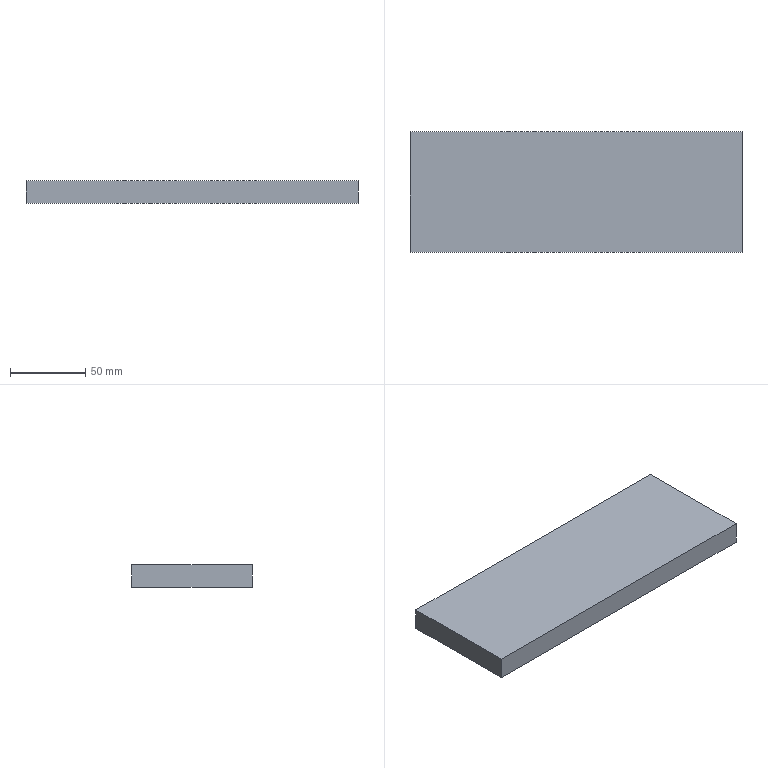Part | STEP file | Tube feed_id586_x_t | 1 solid | 6 faces | box 220 x 80 x 15 mm | volume 264000 mm3 | plane 6
STEP:
#1=CARTESIAN_POINT('',(0.,0.,0.));
#2=DIRECTION('',(0.,0.,1.));
#3=DIRECTION('',(1.,0.,0.));
#4=AXIS2_PLACEMENT_3D('',#1,#2,#3);
#5=CARTESIAN_POINT('',(21.,250.936,-219.));
#6=VERTEX_POINT('',#5);
#7=CARTESIAN_POINT('',(21.,170.936,-219.));
#8=VERTEX_POINT('',#7);
#9=CARTESIAN_POINT('',(21.,250.936,-219.));
#10=DIRECTION('',(0.,-1.,0.));
#11=VECTOR('',#10,1.);
#12=LINE('',#9,#11);
#13=CARTESIAN_POINT('',(21.,250.936,-204.));
#14=DIRECTION('',(1.,0.,0.));
#15=DIRECTION('',(0.,0.,-1.));
#16=AXIS2_PLACEMENT_3D('',#13,#14,#15);
#17=PLANE('',#16);
#18=CARTESIAN_POINT('',(15.,0.));
#19=DIRECTION('',(0.,-1.));
#20=VECTOR('',#19,1.);
#21=LINE('',#18,#20);
#22=(GEOMETRIC_REPRESENTATION_CONTEXT(2)PARAMETRIC_REPRESENTATION_CONTEXT()REPRESENTATION_CONTEXT('',''));
#23=DEFINITIONAL_REPRESENTATION('',(#21),#22);
#24=PCURVE('',#17,#23);
#25=CARTESIAN_POINT('',(0.,0.,-219.));
#26=DIRECTION('',(0.,0.,1.));
#27=DIRECTION('',(1.,0.,0.));
#28=AXIS2_PLACEMENT_3D('',#25,#26,#27);
#29=PLANE('',#28);
#30=CARTESIAN_POINT('',(21.,250.936));
#31=DIRECTION('',(0.,-1.));
#32=VECTOR('',#31,1.);
#33=LINE('',#30,#32);
#34=(GEOMETRIC_REPRESENTATION_CONTEXT(2)PARAMETRIC_REPRESENTATION_CONTEXT()REPRESENTATION_CONTEXT('',''));
#35=DEFINITIONAL_REPRESENTATION('',(#33),#34);
#36=PCURVE('',#29,#35);
#37=SURFACE_CURVE('',#12,(#24,#36),.PCURVE_S1.);
#38=EDGE_CURVE('',#6,#8,#37,.T.);
#39=ORIENTED_EDGE('',*,*,#38,.T.);
#40=CARTESIAN_POINT('',(21.,170.936,-204.));
#41=VERTEX_POINT('',#40);
#42=CARTESIAN_POINT('',(21.,170.936,-204.));
#43=DIRECTION('',(0.,0.,-1.));
#44=VECTOR('',#43,1.);
#45=LINE('',#42,#44);
#46=CARTESIAN_POINT('',(0.,-80.));
#47=DIRECTION('',(1.,0.));
#48=VECTOR('',#47,1.);
#49=LINE('',#46,#48);
#50=(GEOMETRIC_REPRESENTATION_CONTEXT(2)PARAMETRIC_REPRESENTATION_CONTEXT()REPRESENTATION_CONTEXT('',''));
#51=DEFINITIONAL_REPRESENTATION('',(#49),#50);
#52=PCURVE('',#17,#51);
#53=CARTESIAN_POINT('',(21.,170.936,-204.));
#54=DIRECTION('',(0.,1.,0.));
#55=DIRECTION('',(0.,0.,1.));
#56=AXIS2_PLACEMENT_3D('',#53,#54,#55);
#57=PLANE('',#56);
#58=CARTESIAN_POINT('',(0.,0.));
#59=DIRECTION('',(-1.,0.));
#60=VECTOR('',#59,1.);
#61=LINE('',#58,#60);
#62=(GEOMETRIC_REPRESENTATION_CONTEXT(2)PARAMETRIC_REPRESENTATION_CONTEXT()REPRESENTATION_CONTEXT('',''));
#63=DEFINITIONAL_REPRESENTATION('',(#61),#62);
#64=PCURVE('',#57,#63);
#65=SURFACE_CURVE('',#45,(#52,#64),.PCURVE_S1.);
#66=EDGE_CURVE('',#41,#8,#65,.T.);
#67=ORIENTED_EDGE('',*,*,#66,.F.);
#68=CARTESIAN_POINT('',(21.,250.936,-204.));
#69=VERTEX_POINT('',#68);
#70=CARTESIAN_POINT('',(21.,250.936,-204.));
#71=DIRECTION('',(0.,-1.,0.));
#72=VECTOR('',#71,1.);
#73=LINE('',#70,#72);
#74=CARTESIAN_POINT('',(0.,0.));
#75=DIRECTION('',(0.,-1.));
#76=VECTOR('',#75,1.);
#77=LINE('',#74,#76);
#78=(GEOMETRIC_REPRESENTATION_CONTEXT(2)PARAMETRIC_REPRESENTATION_CONTEXT()REPRESENTATION_CONTEXT('',''));
#79=DEFINITIONAL_REPRESENTATION('',(#77),#78);
#80=PCURVE('',#17,#79);
#81=CARTESIAN_POINT('',(0.,0.,-204.));
#82=DIRECTION('',(0.,0.,1.));
#83=DIRECTION('',(1.,0.,0.));
#84=AXIS2_PLACEMENT_3D('',#81,#82,#83);
#85=PLANE('',#84);
#86=CARTESIAN_POINT('',(21.,250.936));
#87=DIRECTION('',(0.,-1.));
#88=VECTOR('',#87,1.);
#89=LINE('',#86,#88);
#90=(GEOMETRIC_REPRESENTATION_CONTEXT(2)PARAMETRIC_REPRESENTATION_CONTEXT()REPRESENTATION_CONTEXT('',''));
#91=DEFINITIONAL_REPRESENTATION('',(#89),#90);
#92=PCURVE('',#85,#91);
#93=SURFACE_CURVE('',#73,(#80,#92),.PCURVE_S1.);
#94=EDGE_CURVE('',#69,#41,#93,.T.);
#95=ORIENTED_EDGE('',*,*,#94,.F.);
#96=CARTESIAN_POINT('',(21.,250.936,-204.));
#97=DIRECTION('',(0.,0.,-1.));
#98=VECTOR('',#97,1.);
#99=LINE('',#96,#98);
#100=CARTESIAN_POINT('',(0.,0.));
#101=DIRECTION('',(1.,0.));
#102=VECTOR('',#101,1.);
#103=LINE('',#100,#102);
#104=(GEOMETRIC_REPRESENTATION_CONTEXT(2)PARAMETRIC_REPRESENTATION_CONTEXT()REPRESENTATION_CONTEXT('',''));
#105=DEFINITIONAL_REPRESENTATION('',(#103),#104);
#106=PCURVE('',#17,#105);
#107=CARTESIAN_POINT('',(241.,250.936,-204.));
#108=DIRECTION('',(0.,-1.,0.));
#109=DIRECTION('',(0.,0.,-1.));
#110=AXIS2_PLACEMENT_3D('',#107,#108,#109);
#111=PLANE('',#110);
#112=CARTESIAN_POINT('',(0.,-220.));
#113=DIRECTION('',(1.,0.));
#114=VECTOR('',#113,1.);
#115=LINE('',#112,#114);
#116=(GEOMETRIC_REPRESENTATION_CONTEXT(2)PARAMETRIC_REPRESENTATION_CONTEXT()REPRESENTATION_CONTEXT('',''));
#117=DEFINITIONAL_REPRESENTATION('',(#115),#116);
#118=PCURVE('',#111,#117);
#119=SURFACE_CURVE('',#99,(#106,#118),.PCURVE_S1.);
#120=EDGE_CURVE('',#69,#6,#119,.T.);
#121=ORIENTED_EDGE('',*,*,#120,.T.);
#122=EDGE_LOOP('',(#39,#67,#95,#121));
#123=FACE_BOUND('',#122,.T.);
#124=ADVANCED_FACE('',(#123),#17,.F.);
#125=CARTESIAN_POINT('',(241.,170.936,-219.));
#126=VERTEX_POINT('',#125);
#127=CARTESIAN_POINT('',(21.,170.936,-219.));
#128=DIRECTION('',(1.,0.,0.));
#129=VECTOR('',#128,1.);
#130=LINE('',#127,#129);
#131=CARTESIAN_POINT('',(-15.,0.));
#132=DIRECTION('',(0.,1.));
#133=VECTOR('',#132,1.);
#134=LINE('',#131,#133);
#135=(GEOMETRIC_REPRESENTATION_CONTEXT(2)PARAMETRIC_REPRESENTATION_CONTEXT()REPRESENTATION_CONTEXT('',''));
#136=DEFINITIONAL_REPRESENTATION('',(#134),#135);
#137=PCURVE('',#57,#136);
#138=CARTESIAN_POINT('',(21.,170.936));
#139=DIRECTION('',(1.,0.));
#140=VECTOR('',#139,1.);
#141=LINE('',#138,#140);
#142=(GEOMETRIC_REPRESENTATION_CONTEXT(2)PARAMETRIC_REPRESENTATION_CONTEXT()REPRESENTATION_CONTEXT('',''));
#143=DEFINITIONAL_REPRESENTATION('',(#141),#142);
#144=PCURVE('',#29,#143);
#145=SURFACE_CURVE('',#130,(#137,#144),.PCURVE_S1.);
#146=EDGE_CURVE('',#8,#126,#145,.T.);
#147=ORIENTED_EDGE('',*,*,#146,.T.);
#148=CARTESIAN_POINT('',(241.,170.936,-204.));
#149=VERTEX_POINT('',#148);
#150=CARTESIAN_POINT('',(241.,170.936,-204.));
#151=DIRECTION('',(0.,0.,-1.));
#152=VECTOR('',#151,1.);
#153=LINE('',#150,#152);
#154=CARTESIAN_POINT('',(0.,220.));
#155=DIRECTION('',(-1.,0.));
#156=VECTOR('',#155,1.);
#157=LINE('',#154,#156);
#158=(GEOMETRIC_REPRESENTATION_CONTEXT(2)PARAMETRIC_REPRESENTATION_CONTEXT()REPRESENTATION_CONTEXT('',''));
#159=DEFINITIONAL_REPRESENTATION('',(#157),#158);
#160=PCURVE('',#57,#159);
#161=CARTESIAN_POINT('',(241.,170.936,-204.));
#162=DIRECTION('',(-1.,0.,0.));
#163=DIRECTION('',(0.,0.,1.));
#164=AXIS2_PLACEMENT_3D('',#161,#162,#163);
#165=PLANE('',#164);
#166=CARTESIAN_POINT('',(0.,0.));
#167=DIRECTION('',(-1.,0.));
#168=VECTOR('',#167,1.);
#169=LINE('',#166,#168);
#170=(GEOMETRIC_REPRESENTATION_CONTEXT(2)PARAMETRIC_REPRESENTATION_CONTEXT()REPRESENTATION_CONTEXT('',''));
#171=DEFINITIONAL_REPRESENTATION('',(#169),#170);
#172=PCURVE('',#165,#171);
#173=SURFACE_CURVE('',#153,(#160,#172),.PCURVE_S1.);
#174=EDGE_CURVE('',#149,#126,#173,.T.);
#175=ORIENTED_EDGE('',*,*,#174,.F.);
#176=CARTESIAN_POINT('',(21.,170.936,-204.));
#177=DIRECTION('',(1.,0.,0.));
#178=VECTOR('',#177,1.);
#179=LINE('',#176,#178);
#180=CARTESIAN_POINT('',(0.,0.));
#181=DIRECTION('',(0.,1.));
#182=VECTOR('',#181,1.);
#183=LINE('',#180,#182);
#184=(GEOMETRIC_REPRESENTATION_CONTEXT(2)PARAMETRIC_REPRESENTATION_CONTEXT()REPRESENTATION_CONTEXT('',''));
#185=DEFINITIONAL_REPRESENTATION('',(#183),#184);
#186=PCURVE('',#57,#185);
#187=CARTESIAN_POINT('',(21.,170.936));
#188=DIRECTION('',(1.,0.));
#189=VECTOR('',#188,1.);
#190=LINE('',#187,#189);
#191=(GEOMETRIC_REPRESENTATION_CONTEXT(2)PARAMETRIC_REPRESENTATION_CONTEXT()REPRESENTATION_CONTEXT('',''));
#192=DEFINITIONAL_REPRESENTATION('',(#190),#191);
#193=PCURVE('',#85,#192);
#194=SURFACE_CURVE('',#179,(#186,#193),.PCURVE_S1.);
#195=EDGE_CURVE('',#41,#149,#194,.T.);
#196=ORIENTED_EDGE('',*,*,#195,.F.);
#197=ORIENTED_EDGE('',*,*,#66,.T.);
#198=EDGE_LOOP('',(#147,#175,#196,#197));
#199=FACE_BOUND('',#198,.T.);
#200=ADVANCED_FACE('',(#199),#57,.F.);
#201=CARTESIAN_POINT('',(241.,250.936,-219.));
#202=VERTEX_POINT('',#201);
#203=CARTESIAN_POINT('',(241.,170.936,-219.));
#204=DIRECTION('',(0.,1.,0.));
#205=VECTOR('',#204,1.);
#206=LINE('',#203,#205);
#207=CARTESIAN_POINT('',(-15.,0.));
#208=DIRECTION('',(0.,1.));
#209=VECTOR('',#208,1.);
#210=LINE('',#207,#209);
#211=(GEOMETRIC_REPRESENTATION_CONTEXT(2)PARAMETRIC_REPRESENTATION_CONTEXT()REPRESENTATION_CONTEXT('',''));
#212=DEFINITIONAL_REPRESENTATION('',(#210),#211);
#213=PCURVE('',#165,#212);
#214=CARTESIAN_POINT('',(241.,170.936));
#215=DIRECTION('',(0.,1.));
#216=VECTOR('',#215,1.);
#217=LINE('',#214,#216);
#218=(GEOMETRIC_REPRESENTATION_CONTEXT(2)PARAMETRIC_REPRESENTATION_CONTEXT()REPRESENTATION_CONTEXT('',''));
#219=DEFINITIONAL_REPRESENTATION('',(#217),#218);
#220=PCURVE('',#29,#219);
#221=SURFACE_CURVE('',#206,(#213,#220),.PCURVE_S1.);
#222=EDGE_CURVE('',#126,#202,#221,.T.);
#223=ORIENTED_EDGE('',*,*,#222,.T.);
#224=CARTESIAN_POINT('',(241.,250.936,-204.));
#225=VERTEX_POINT('',#224);
#226=CARTESIAN_POINT('',(241.,250.936,-204.));
#227=DIRECTION('',(0.,0.,-1.));
#228=VECTOR('',#227,1.);
#229=LINE('',#226,#228);
#230=CARTESIAN_POINT('',(0.,80.));
#231=DIRECTION('',(-1.,0.));
#232=VECTOR('',#231,1.);
#233=LINE('',#230,#232);
#234=(GEOMETRIC_REPRESENTATION_CONTEXT(2)PARAMETRIC_REPRESENTATION_CONTEXT()REPRESENTATION_CONTEXT('',''));
#235=DEFINITIONAL_REPRESENTATION('',(#233),#234);
#236=PCURVE('',#165,#235);
#237=CARTESIAN_POINT('',(0.,0.));
#238=DIRECTION('',(1.,0.));
#239=VECTOR('',#238,1.);
#240=LINE('',#237,#239);
#241=(GEOMETRIC_REPRESENTATION_CONTEXT(2)PARAMETRIC_REPRESENTATION_CONTEXT()REPRESENTATION_CONTEXT('',''));
#242=DEFINITIONAL_REPRESENTATION('',(#240),#241);
#243=PCURVE('',#111,#242);
#244=SURFACE_CURVE('',#229,(#236,#243),.PCURVE_S1.);
#245=EDGE_CURVE('',#225,#202,#244,.T.);
#246=ORIENTED_EDGE('',*,*,#245,.F.);
#247=CARTESIAN_POINT('',(241.,170.936,-204.));
#248=DIRECTION('',(0.,1.,0.));
#249=VECTOR('',#248,1.);
#250=LINE('',#247,#249);
#251=CARTESIAN_POINT('',(0.,0.));
#252=DIRECTION('',(0.,1.));
#253=VECTOR('',#252,1.);
#254=LINE('',#251,#253);
#255=(GEOMETRIC_REPRESENTATION_CONTEXT(2)PARAMETRIC_REPRESENTATION_CONTEXT()REPRESENTATION_CONTEXT('',''));
#256=DEFINITIONAL_REPRESENTATION('',(#254),#255);
#257=PCURVE('',#165,#256);
#258=CARTESIAN_POINT('',(241.,170.936));
#259=DIRECTION('',(0.,1.));
#260=VECTOR('',#259,1.);
#261=LINE('',#258,#260);
#262=(GEOMETRIC_REPRESENTATION_CONTEXT(2)PARAMETRIC_REPRESENTATION_CONTEXT()REPRESENTATION_CONTEXT('',''));
#263=DEFINITIONAL_REPRESENTATION('',(#261),#262);
#264=PCURVE('',#85,#263);
#265=SURFACE_CURVE('',#250,(#257,#264),.PCURVE_S1.);
#266=EDGE_CURVE('',#149,#225,#265,.T.);
#267=ORIENTED_EDGE('',*,*,#266,.F.);
#268=ORIENTED_EDGE('',*,*,#174,.T.);
#269=EDGE_LOOP('',(#223,#246,#267,#268));
#270=FACE_BOUND('',#269,.T.);
#271=ADVANCED_FACE('',(#270),#165,.F.);
#272=CARTESIAN_POINT('',(241.,250.936,-219.));
#273=DIRECTION('',(-1.,0.,0.));
#274=VECTOR('',#273,1.);
#275=LINE('',#272,#274);
#276=CARTESIAN_POINT('',(15.,0.));
#277=DIRECTION('',(0.,-1.));
#278=VECTOR('',#277,1.);
#279=LINE('',#276,#278);
#280=(GEOMETRIC_REPRESENTATION_CONTEXT(2)PARAMETRIC_REPRESENTATION_CONTEXT()REPRESENTATION_CONTEXT('',''));
#281=DEFINITIONAL_REPRESENTATION('',(#279),#280);
#282=PCURVE('',#111,#281);
#283=CARTESIAN_POINT('',(241.,250.936));
#284=DIRECTION('',(-1.,0.));
#285=VECTOR('',#284,1.);
#286=LINE('',#283,#285);
#287=(GEOMETRIC_REPRESENTATION_CONTEXT(2)PARAMETRIC_REPRESENTATION_CONTEXT()REPRESENTATION_CONTEXT('',''));
#288=DEFINITIONAL_REPRESENTATION('',(#286),#287);
#289=PCURVE('',#29,#288);
#290=SURFACE_CURVE('',#275,(#282,#289),.PCURVE_S1.);
#291=EDGE_CURVE('',#202,#6,#290,.T.);
#292=ORIENTED_EDGE('',*,*,#291,.T.);
#293=ORIENTED_EDGE('',*,*,#120,.F.);
#294=CARTESIAN_POINT('',(241.,250.936,-204.));
#295=DIRECTION('',(-1.,0.,0.));
#296=VECTOR('',#295,1.);
#297=LINE('',#294,#296);
#298=CARTESIAN_POINT('',(0.,0.));
#299=DIRECTION('',(0.,-1.));
#300=VECTOR('',#299,1.);
#301=LINE('',#298,#300);
#302=(GEOMETRIC_REPRESENTATION_CONTEXT(2)PARAMETRIC_REPRESENTATION_CONTEXT()REPRESENTATION_CONTEXT('',''));
#303=DEFINITIONAL_REPRESENTATION('',(#301),#302);
#304=PCURVE('',#111,#303);
#305=CARTESIAN_POINT('',(241.,250.936));
#306=DIRECTION('',(-1.,0.));
#307=VECTOR('',#306,1.);
#308=LINE('',#305,#307);
#309=(GEOMETRIC_REPRESENTATION_CONTEXT(2)PARAMETRIC_REPRESENTATION_CONTEXT()REPRESENTATION_CONTEXT('',''));
#310=DEFINITIONAL_REPRESENTATION('',(#308),#309);
#311=PCURVE('',#85,#310);
#312=SURFACE_CURVE('',#297,(#304,#311),.PCURVE_S1.);
#313=EDGE_CURVE('',#225,#69,#312,.T.);
#314=ORIENTED_EDGE('',*,*,#313,.F.);
#315=ORIENTED_EDGE('',*,*,#245,.T.);
#316=EDGE_LOOP('',(#292,#293,#314,#315));
#317=FACE_BOUND('',#316,.T.);
#318=ADVANCED_FACE('',(#317),#111,.F.);
#319=ORIENTED_EDGE('',*,*,#94,.T.);
#320=ORIENTED_EDGE('',*,*,#195,.T.);
#321=ORIENTED_EDGE('',*,*,#266,.T.);
#322=ORIENTED_EDGE('',*,*,#313,.T.);
#323=EDGE_LOOP('',(#319,#320,#321,#322));
#324=FACE_BOUND('',#323,.T.);
#325=ADVANCED_FACE('',(#324),#85,.T.);
#326=ORIENTED_EDGE('',*,*,#38,.F.);
#327=ORIENTED_EDGE('',*,*,#291,.F.);
#328=ORIENTED_EDGE('',*,*,#222,.F.);
#329=ORIENTED_EDGE('',*,*,#146,.F.);
#330=EDGE_LOOP('',(#326,#327,#328,#329));
#331=FACE_BOUND('',#330,.T.);
#332=ADVANCED_FACE('',(#331),#29,.F.);
#333=CLOSED_SHELL('',(#124,#200,#271,#318,#325,#332));
#334=MANIFOLD_SOLID_BREP('',#333);
#335=(LENGTH_UNIT()NAMED_UNIT(*)SI_UNIT(.MILLI.,.METRE.));
#336=UNCERTAINTY_MEASURE_WITH_UNIT(LENGTH_MEASURE(0.0000001),#335,'','');
#337=(NAMED_UNIT(*)PLANE_ANGLE_UNIT()SI_UNIT($,.RADIAN.));
#338=(NAMED_UNIT(*)SI_UNIT($,.STERADIAN.)SOLID_ANGLE_UNIT());
#339=(GEOMETRIC_REPRESENTATION_CONTEXT(3)GLOBAL_UNCERTAINTY_ASSIGNED_CONTEXT((#336))GLOBAL_UNIT_ASSIGNED_CONTEXT((#335,#337,#338))REPRESENTATION_CONTEXT('',''));
#340=ADVANCED_BREP_SHAPE_REPRESENTATION('',(#4,#334),#339);